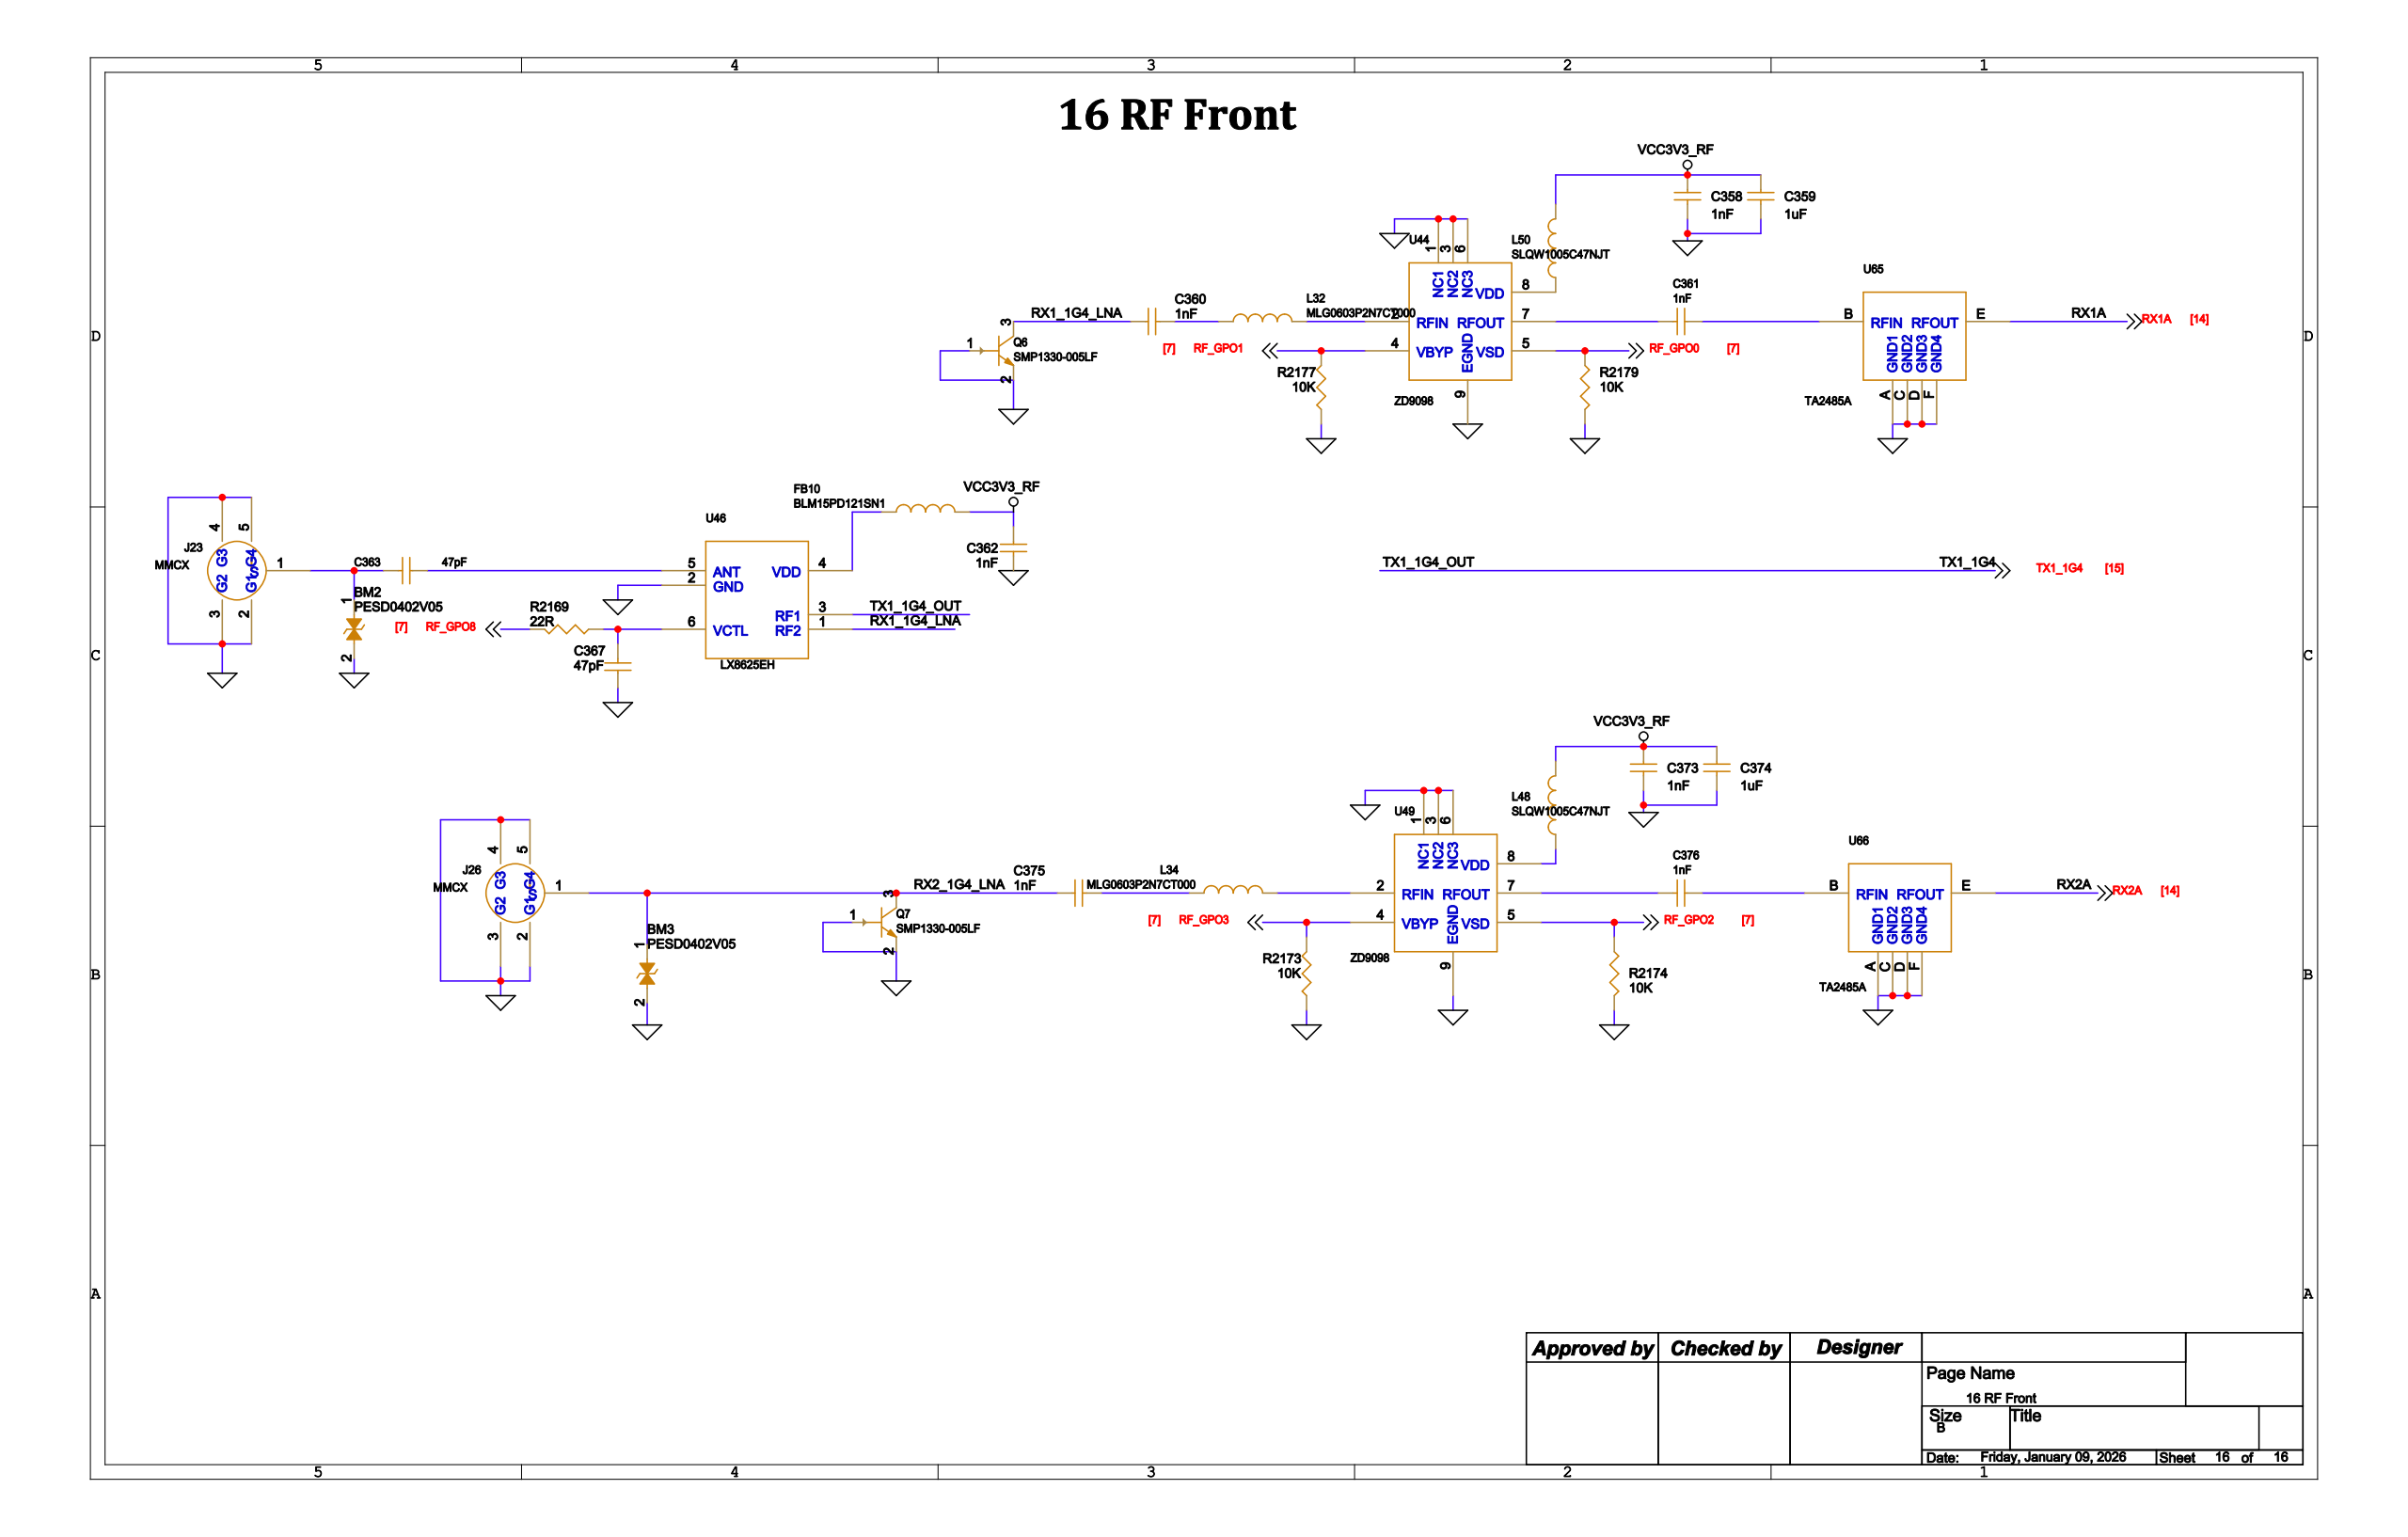Circuit board | Cadence Allegro | 442 parts | 326 nets | one sheet of the schematic
Parts on this sheet (reference | value | footprint):
BM2 | PESD0402V05 | TVS0402
BM3 | PESD0402V05 | TVS0402
C358 | 1nF | C0201
C359 | 1uF | C0201
C360 | 1nF | C0201
C361 | 1nF | C0201
C362 | 1nF | C0201
C363 | 47pF | C0402_D
C367 | 47pF | C0402_D
C373 | 1nF | C0201
C374 | 1uF | C0201
C375 | 1nF | C0201
C376 | 1nF | C0201
FB10 | BLM15PD121SN1 | L0402_D
J23 | MMCX | DL-MMCX-KWE-90
J26 | MMCX | DL-MMCX-KWE-90
L32 | MLG0603P2N7CT000 | L0201
L34 | MLG0603P2N7CT000 | L0402_D
L48 | SLQW1005C47NJT | L0402_D
L50 | SLQW1005C47NJT | L0402_D
Q6 | SMP1330-005LF | SOT-23
Q7 | SMP1330-005LF | SOT-23
R2169 | 22R | R0201
R2173 | 10K | R0201
R2174 | 10K | R0201
R2177 | 10K | R0201
R2179 | 10K | R0201
U44 | ZD9098 | DFN2X2-8P
U46 | LX8625EH | DFN6_1_1_0_7MM
U49 | ZD9098 | DFN2X2-8P
U65 | TA2485A | TA2494A
U66 | TA2485A | TA2494A
Nets of these parts (net: part-pin ...):
GND: BM2-2 BM3-2 C358-2 C359-2 C362-2 C367-1 C373-2 C374-2 J23-2 J23-3 J23-4 J23-5 J26-2 J26-3 J26-4 J26-5 Q6-1 Q6-2 Q7-1 Q7-2 R2173-1 R2174-2 R2177-1 R2179-2 U44-1 U44-3 U44-6 U44-9 U46-2 U49-1 U49-3 U49-6 U49-9 U65-A U65-C U65-D U65-F U66-A U66-C U66-D U66-F
N49088438: BM2-1 C363-2 J23-1
RX2_1G4_LNA: BM3-1 C375-1 J26-1 Q7-3
RX1_1G4_LNA: C360-1 Q6-3 U46-1
VCC3V3_RF: C358-1 C359-1 C362-1 C373-1 C374-1 FB10-2 L48-2 L50-2
N38188746: C363-1 U46-5
N50020375: C367-2 R2169-2 U46-6
N49193940: C360-2 L32-1
N49181397: L32-2 U44-2
N50289007: C375-2 L34-1
N49181793: L34-2 U49-2
N50084496: L48-1 U49-8
N505312978: L50-1 U44-8
RF_GPO8: R2169-1
N50025513: C361-1 U65-B
RX1A: U65-E
N50058764: C376-1 U66-B
RX2A: U66-E
N50025516: C361-2 U44-7
RF_GPO1: R2177-2 U44-4
RF_GPO0: R2179-1 U44-5
N49181807: C376-2 U49-7
RF_GPO3: R2173-2 U49-4
RF_GPO2: R2174-1 U49-5
TX1_1G4: U46-3
N49090908: FB10-1 U46-4